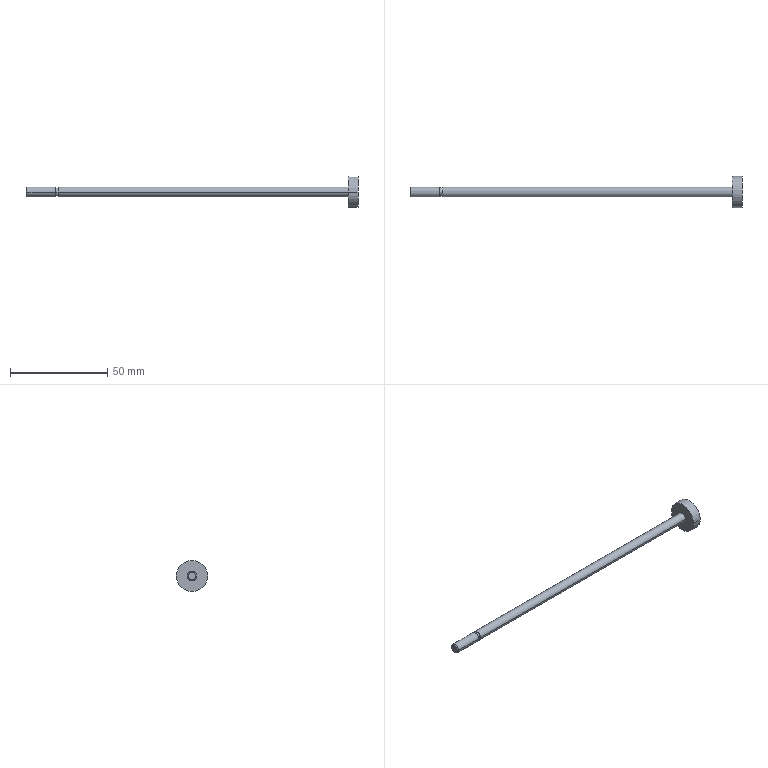Part | SolidWorks | features RefAxis 9, 3DProfileFeature 3, Revolution 1 | 1 solid | 15 faces | box 170.5 x 16 x 16 mm | volume 4244 mm3 | cylinder 8 | plane 5 | cone 2 | commonest cylinder face diameters 5 x4 4.134 x2 16 x2
STEP:
#1=CARTESIAN_POINT('',(170.5,-8.,0.));
#2=VERTEX_POINT('',#1);
#3=CARTESIAN_POINT('',(170.5,8.,0.));
#4=VERTEX_POINT('',#3);
#5=CARTESIAN_POINT('',(170.5,0.,0.));
#6=DIRECTION('',(-1.,0.,0.));
#7=DIRECTION('',(0.,-1.,0.));
#8=AXIS2_PLACEMENT_3D('',#5,#6,#7);
#9=CIRCLE('',#8,8.);
#10=EDGE_CURVE('',#2,#4,#9,.T.);
#11=ORIENTED_EDGE('',*,*,#10,.T.);
#12=CARTESIAN_POINT('',(165.5,8.,0.));
#13=VERTEX_POINT('',#12);
#14=CARTESIAN_POINT('',(170.5,8.,0.));
#15=DIRECTION('',(-1.,0.,0.));
#16=VECTOR('',#15,1000.);
#17=LINE('',#14,#16);
#18=EDGE_CURVE('',#4,#13,#17,.T.);
#19=ORIENTED_EDGE('',*,*,#18,.T.);
#20=CARTESIAN_POINT('',(165.5,-8.,0.));
#21=VERTEX_POINT('',#20);
#22=CARTESIAN_POINT('',(165.5,0.,0.));
#23=DIRECTION('',(-1.,0.,0.));
#24=DIRECTION('',(0.,-1.,0.));
#25=AXIS2_PLACEMENT_3D('',#22,#23,#24);
#26=CIRCLE('',#25,8.);
#27=EDGE_CURVE('',#21,#13,#26,.T.);
#28=ORIENTED_EDGE('',*,*,#27,.F.);
#29=CARTESIAN_POINT('',(170.5,-8.,0.));
#30=DIRECTION('',(-1.,0.,0.));
#31=VECTOR('',#30,1000.);
#32=LINE('',#29,#31);
#33=EDGE_CURVE('',#2,#21,#32,.T.);
#34=ORIENTED_EDGE('',*,*,#33,.F.);
#35=EDGE_LOOP('',(#11,#19,#28,#34));
#36=FACE_OUTER_BOUND('',#35,.T.);
#37=CARTESIAN_POINT('',(170.5,0.,0.));
#38=DIRECTION('',(-1.,0.,0.));
#39=DIRECTION('',(0.,-1.,0.));
#40=AXIS2_PLACEMENT_3D('',#37,#38,#39);
#41=CYLINDRICAL_SURFACE('',#40,8.);
#42=ADVANCED_FACE('',(#36),#41,.T.);
#43=CARTESIAN_POINT('',(165.5,-2.5,0.));
#44=VERTEX_POINT('',#43);
#45=CARTESIAN_POINT('',(165.5,2.5,0.));
#46=VERTEX_POINT('',#45);
#47=CARTESIAN_POINT('',(165.5,0.,0.));
#48=DIRECTION('',(-1.,0.,0.));
#49=DIRECTION('',(0.,-1.,0.));
#50=AXIS2_PLACEMENT_3D('',#47,#48,#49);
#51=CIRCLE('',#50,2.5);
#52=EDGE_CURVE('',#44,#46,#51,.T.);
#53=ORIENTED_EDGE('',*,*,#52,.T.);
#54=CARTESIAN_POINT('',(16.5,2.5,0.));
#55=VERTEX_POINT('',#54);
#56=CARTESIAN_POINT('',(170.5,2.5,0.));
#57=DIRECTION('',(-1.,0.,0.));
#58=VECTOR('',#57,1000.);
#59=LINE('',#56,#58);
#60=EDGE_CURVE('',#46,#55,#59,.T.);
#61=ORIENTED_EDGE('',*,*,#60,.T.);
#62=CARTESIAN_POINT('',(16.5,-2.5,0.));
#63=VERTEX_POINT('',#62);
#64=CARTESIAN_POINT('',(16.5,0.,0.));
#65=DIRECTION('',(-1.,0.,0.));
#66=DIRECTION('',(0.,-1.,0.));
#67=AXIS2_PLACEMENT_3D('',#64,#65,#66);
#68=CIRCLE('',#67,2.5);
#69=EDGE_CURVE('',#63,#55,#68,.T.);
#70=ORIENTED_EDGE('',*,*,#69,.F.);
#71=CARTESIAN_POINT('',(170.5,-2.5,0.));
#72=DIRECTION('',(-1.,0.,0.));
#73=VECTOR('',#72,1000.);
#74=LINE('',#71,#73);
#75=EDGE_CURVE('',#44,#63,#74,.T.);
#76=ORIENTED_EDGE('',*,*,#75,.F.);
#77=EDGE_LOOP('',(#53,#61,#70,#76));
#78=FACE_OUTER_BOUND('',#77,.T.);
#79=CARTESIAN_POINT('',(170.5,0.,0.));
#80=DIRECTION('',(-1.,0.,0.));
#81=DIRECTION('',(0.,-1.,0.));
#82=AXIS2_PLACEMENT_3D('',#79,#80,#81);
#83=CYLINDRICAL_SURFACE('',#82,2.5);
#84=ADVANCED_FACE('',(#78),#83,.T.);
#85=CARTESIAN_POINT('',(16.5,-2.067,0.));
#86=VERTEX_POINT('',#85);
#87=CARTESIAN_POINT('',(16.5,2.067,0.));
#88=VERTEX_POINT('',#87);
#89=CARTESIAN_POINT('',(16.5,0.,0.));
#90=DIRECTION('',(-1.,0.,0.));
#91=DIRECTION('',(0.,-1.,0.));
#92=AXIS2_PLACEMENT_3D('',#89,#90,#91);
#93=CIRCLE('',#92,2.067);
#94=EDGE_CURVE('',#86,#88,#93,.T.);
#95=ORIENTED_EDGE('',*,*,#94,.T.);
#96=CARTESIAN_POINT('',(15.,2.067,0.));
#97=VERTEX_POINT('',#96);
#98=CARTESIAN_POINT('',(170.5,2.067,0.));
#99=DIRECTION('',(-1.,0.,0.));
#100=VECTOR('',#99,1000.);
#101=LINE('',#98,#100);
#102=EDGE_CURVE('',#88,#97,#101,.T.);
#103=ORIENTED_EDGE('',*,*,#102,.T.);
#104=CARTESIAN_POINT('',(15.,-2.067,0.));
#105=VERTEX_POINT('',#104);
#106=CARTESIAN_POINT('',(15.,0.,0.));
#107=DIRECTION('',(-1.,0.,0.));
#108=DIRECTION('',(0.,-1.,0.));
#109=AXIS2_PLACEMENT_3D('',#106,#107,#108);
#110=CIRCLE('',#109,2.067);
#111=EDGE_CURVE('',#105,#97,#110,.T.);
#112=ORIENTED_EDGE('',*,*,#111,.F.);
#113=CARTESIAN_POINT('',(170.5,-2.067,0.));
#114=DIRECTION('',(-1.,0.,0.));
#115=VECTOR('',#114,1000.);
#116=LINE('',#113,#115);
#117=EDGE_CURVE('',#86,#105,#116,.T.);
#118=ORIENTED_EDGE('',*,*,#117,.F.);
#119=EDGE_LOOP('',(#95,#103,#112,#118));
#120=FACE_OUTER_BOUND('',#119,.T.);
#121=CARTESIAN_POINT('',(170.5,0.,0.));
#122=DIRECTION('',(-1.,0.,0.));
#123=DIRECTION('',(0.,-1.,0.));
#124=AXIS2_PLACEMENT_3D('',#121,#122,#123);
#125=CYLINDRICAL_SURFACE('',#124,2.067);
#126=ADVANCED_FACE('',(#120),#125,.T.);
#127=CARTESIAN_POINT('',(15.,-2.5,0.));
#128=VERTEX_POINT('',#127);
#129=CARTESIAN_POINT('',(15.,2.5,0.));
#130=VERTEX_POINT('',#129);
#131=CARTESIAN_POINT('',(15.,0.,0.));
#132=DIRECTION('',(-1.,0.,0.));
#133=DIRECTION('',(0.,-1.,0.));
#134=AXIS2_PLACEMENT_3D('',#131,#132,#133);
#135=CIRCLE('',#134,2.5);
#136=EDGE_CURVE('',#128,#130,#135,.T.);
#137=ORIENTED_EDGE('',*,*,#136,.T.);
#138=CARTESIAN_POINT('',(0.4905,2.5,0.));
#139=VERTEX_POINT('',#138);
#140=CARTESIAN_POINT('',(170.5,2.5,0.));
#141=DIRECTION('',(-1.,0.,0.));
#142=VECTOR('',#141,1000.);
#143=LINE('',#140,#142);
#144=EDGE_CURVE('',#130,#139,#143,.T.);
#145=ORIENTED_EDGE('',*,*,#144,.T.);
#146=CARTESIAN_POINT('',(0.4905,-2.5,0.));
#147=VERTEX_POINT('',#146);
#148=CARTESIAN_POINT('',(0.4905,0.,0.));
#149=DIRECTION('',(-1.,0.,0.));
#150=DIRECTION('',(0.,-1.,0.));
#151=AXIS2_PLACEMENT_3D('',#148,#149,#150);
#152=CIRCLE('',#151,2.5);
#153=EDGE_CURVE('',#147,#139,#152,.T.);
#154=ORIENTED_EDGE('',*,*,#153,.F.);
#155=CARTESIAN_POINT('',(170.5,-2.5,0.));
#156=DIRECTION('',(-1.,0.,0.));
#157=VECTOR('',#156,1000.);
#158=LINE('',#155,#157);
#159=EDGE_CURVE('',#128,#147,#158,.T.);
#160=ORIENTED_EDGE('',*,*,#159,.F.);
#161=EDGE_LOOP('',(#137,#145,#154,#160));
#162=FACE_OUTER_BOUND('',#161,.T.);
#163=CARTESIAN_POINT('',(170.5,0.,0.));
#164=DIRECTION('',(-1.,0.,0.));
#165=DIRECTION('',(0.,-1.,0.));
#166=AXIS2_PLACEMENT_3D('',#163,#164,#165);
#167=CYLINDRICAL_SURFACE('',#166,2.5);
#168=ADVANCED_FACE('',(#162),#167,.T.);
#169=CARTESIAN_POINT('',(0.,-2.01,0.));
#170=VERTEX_POINT('',#169);
#171=CARTESIAN_POINT('',(0.,2.01,0.));
#172=VERTEX_POINT('',#171);
#173=CARTESIAN_POINT('',(0.,0.,0.));
#174=DIRECTION('',(-1.,0.,0.));
#175=DIRECTION('',(0.,-1.,0.));
#176=AXIS2_PLACEMENT_3D('',#173,#174,#175);
#177=CIRCLE('',#176,2.01);
#178=EDGE_CURVE('',#170,#172,#177,.T.);
#179=ORIENTED_EDGE('',*,*,#178,.F.);
#180=CARTESIAN_POINT('',(0.4905,-2.5,0.));
#181=DIRECTION('',(0.7071,-0.7071,0.));
#182=VECTOR('',#181,1000.);
#183=LINE('',#180,#182);
#184=EDGE_CURVE('',#170,#147,#183,.T.);
#185=ORIENTED_EDGE('',*,*,#184,.T.);
#186=ORIENTED_EDGE('',*,*,#153,.T.);
#187=CARTESIAN_POINT('',(0.4905,2.5,0.));
#188=DIRECTION('',(0.7071,0.7071,0.));
#189=VECTOR('',#188,1000.);
#190=LINE('',#187,#189);
#191=EDGE_CURVE('',#172,#139,#190,.T.);
#192=ORIENTED_EDGE('',*,*,#191,.F.);
#193=EDGE_LOOP('',(#179,#185,#186,#192));
#194=FACE_OUTER_BOUND('',#193,.T.);
#195=CARTESIAN_POINT('',(0.4905,0.,0.));
#196=DIRECTION('',(1.,0.,0.));
#197=DIRECTION('',(0.,1.,0.));
#198=AXIS2_PLACEMENT_3D('',#195,#196,#197);
#199=CONICAL_SURFACE('',#198,2.5,0.7854);
#200=ADVANCED_FACE('',(#194),#199,.T.);
#201=CARTESIAN_POINT('',(0.,0.,0.));
#202=DIRECTION('',(-1.,0.,0.));
#203=DIRECTION('',(0.,-1.,0.));
#204=AXIS2_PLACEMENT_3D('',#201,#202,#203);
#205=CIRCLE('',#204,2.01);
#206=EDGE_CURVE('',#172,#170,#205,.T.);
#207=ORIENTED_EDGE('',*,*,#206,.T.);
#208=ORIENTED_EDGE('',*,*,#178,.T.);
#209=EDGE_LOOP('',(#207,#208));
#210=FACE_OUTER_BOUND('',#209,.T.);
#211=CARTESIAN_POINT('',(0.,0.,0.));
#212=DIRECTION('',(1.,0.,0.));
#213=DIRECTION('',(0.,1.,0.));
#214=AXIS2_PLACEMENT_3D('',#211,#212,#213);
#215=PLANE('',#214);
#216=ADVANCED_FACE('',(#210),#215,.F.);
#217=ORIENTED_EDGE('',*,*,#184,.F.);
#218=ORIENTED_EDGE('',*,*,#206,.F.);
#219=ORIENTED_EDGE('',*,*,#191,.T.);
#220=CARTESIAN_POINT('',(0.4905,0.,0.));
#221=DIRECTION('',(-1.,0.,0.));
#222=DIRECTION('',(0.,-1.,0.));
#223=AXIS2_PLACEMENT_3D('',#220,#221,#222);
#224=CIRCLE('',#223,2.5);
#225=EDGE_CURVE('',#139,#147,#224,.T.);
#226=ORIENTED_EDGE('',*,*,#225,.T.);
#227=EDGE_LOOP('',(#217,#218,#219,#226));
#228=FACE_OUTER_BOUND('',#227,.T.);
#229=CARTESIAN_POINT('',(0.4905,0.,0.));
#230=DIRECTION('',(1.,0.,0.));
#231=DIRECTION('',(0.,1.,0.));
#232=AXIS2_PLACEMENT_3D('',#229,#230,#231);
#233=CONICAL_SURFACE('',#232,2.5,0.7854);
#234=ADVANCED_FACE('',(#228),#233,.T.);
#235=ORIENTED_EDGE('',*,*,#144,.F.);
#236=CARTESIAN_POINT('',(15.,0.,0.));
#237=DIRECTION('',(-1.,0.,0.));
#238=DIRECTION('',(0.,-1.,0.));
#239=AXIS2_PLACEMENT_3D('',#236,#237,#238);
#240=CIRCLE('',#239,2.5);
#241=EDGE_CURVE('',#130,#128,#240,.T.);
#242=ORIENTED_EDGE('',*,*,#241,.T.);
#243=ORIENTED_EDGE('',*,*,#159,.T.);
#244=ORIENTED_EDGE('',*,*,#225,.F.);
#245=EDGE_LOOP('',(#235,#242,#243,#244));
#246=FACE_OUTER_BOUND('',#245,.T.);
#247=CARTESIAN_POINT('',(170.5,0.,0.));
#248=DIRECTION('',(-1.,0.,0.));
#249=DIRECTION('',(0.,-1.,0.));
#250=AXIS2_PLACEMENT_3D('',#247,#248,#249);
#251=CYLINDRICAL_SURFACE('',#250,2.5);
#252=ADVANCED_FACE('',(#246),#251,.T.);
#253=ORIENTED_EDGE('',*,*,#136,.F.);
#254=ORIENTED_EDGE('',*,*,#241,.F.);
#255=EDGE_LOOP('',(#253,#254));
#256=FACE_OUTER_BOUND('',#255,.T.);
#257=ORIENTED_EDGE('',*,*,#111,.T.);
#258=CARTESIAN_POINT('',(15.,0.,0.));
#259=DIRECTION('',(-1.,0.,0.));
#260=DIRECTION('',(0.,-1.,0.));
#261=AXIS2_PLACEMENT_3D('',#258,#259,#260);
#262=CIRCLE('',#261,2.067);
#263=EDGE_CURVE('',#97,#105,#262,.T.);
#264=ORIENTED_EDGE('',*,*,#263,.T.);
#265=EDGE_LOOP('',(#257,#264));
#266=FACE_BOUND('',#265,.T.);
#267=CARTESIAN_POINT('',(15.,2.5,0.));
#268=DIRECTION('',(-1.,0.,0.));
#269=DIRECTION('',(0.,-1.,0.));
#270=AXIS2_PLACEMENT_3D('',#267,#268,#269);
#271=PLANE('',#270);
#272=ADVANCED_FACE('',(#256,#266),#271,.F.);
#273=ORIENTED_EDGE('',*,*,#102,.F.);
#274=CARTESIAN_POINT('',(16.5,0.,0.));
#275=DIRECTION('',(-1.,0.,0.));
#276=DIRECTION('',(0.,-1.,0.));
#277=AXIS2_PLACEMENT_3D('',#274,#275,#276);
#278=CIRCLE('',#277,2.067);
#279=EDGE_CURVE('',#88,#86,#278,.T.);
#280=ORIENTED_EDGE('',*,*,#279,.T.);
#281=ORIENTED_EDGE('',*,*,#117,.T.);
#282=ORIENTED_EDGE('',*,*,#263,.F.);
#283=EDGE_LOOP('',(#273,#280,#281,#282));
#284=FACE_OUTER_BOUND('',#283,.T.);
#285=CARTESIAN_POINT('',(170.5,0.,0.));
#286=DIRECTION('',(-1.,0.,0.));
#287=DIRECTION('',(0.,-1.,0.));
#288=AXIS2_PLACEMENT_3D('',#285,#286,#287);
#289=CYLINDRICAL_SURFACE('',#288,2.067);
#290=ADVANCED_FACE('',(#284),#289,.T.);
#291=ORIENTED_EDGE('',*,*,#94,.F.);
#292=ORIENTED_EDGE('',*,*,#279,.F.);
#293=EDGE_LOOP('',(#291,#292));
#294=FACE_BOUND('',#293,.T.);
#295=ORIENTED_EDGE('',*,*,#69,.T.);
#296=CARTESIAN_POINT('',(16.5,0.,0.));
#297=DIRECTION('',(-1.,0.,0.));
#298=DIRECTION('',(0.,-1.,0.));
#299=AXIS2_PLACEMENT_3D('',#296,#297,#298);
#300=CIRCLE('',#299,2.5);
#301=EDGE_CURVE('',#55,#63,#300,.T.);
#302=ORIENTED_EDGE('',*,*,#301,.T.);
#303=EDGE_LOOP('',(#295,#302));
#304=FACE_OUTER_BOUND('',#303,.T.);
#305=CARTESIAN_POINT('',(16.5,2.067,0.));
#306=DIRECTION('',(1.,0.,0.));
#307=DIRECTION('',(0.,1.,0.));
#308=AXIS2_PLACEMENT_3D('',#305,#306,#307);
#309=PLANE('',#308);
#310=ADVANCED_FACE('',(#294,#304),#309,.F.);
#311=ORIENTED_EDGE('',*,*,#60,.F.);
#312=CARTESIAN_POINT('',(165.5,0.,0.));
#313=DIRECTION('',(-1.,0.,0.));
#314=DIRECTION('',(0.,-1.,0.));
#315=AXIS2_PLACEMENT_3D('',#312,#313,#314);
#316=CIRCLE('',#315,2.5);
#317=EDGE_CURVE('',#46,#44,#316,.T.);
#318=ORIENTED_EDGE('',*,*,#317,.T.);
#319=ORIENTED_EDGE('',*,*,#75,.T.);
#320=ORIENTED_EDGE('',*,*,#301,.F.);
#321=EDGE_LOOP('',(#311,#318,#319,#320));
#322=FACE_OUTER_BOUND('',#321,.T.);
#323=CARTESIAN_POINT('',(170.5,0.,0.));
#324=DIRECTION('',(-1.,0.,0.));
#325=DIRECTION('',(0.,-1.,0.));
#326=AXIS2_PLACEMENT_3D('',#323,#324,#325);
#327=CYLINDRICAL_SURFACE('',#326,2.5);
#328=ADVANCED_FACE('',(#322),#327,.T.);
#329=ORIENTED_EDGE('',*,*,#52,.F.);
#330=ORIENTED_EDGE('',*,*,#317,.F.);
#331=EDGE_LOOP('',(#329,#330));
#332=FACE_BOUND('',#331,.T.);
#333=ORIENTED_EDGE('',*,*,#27,.T.);
#334=CARTESIAN_POINT('',(165.5,0.,0.));
#335=DIRECTION('',(-1.,0.,0.));
#336=DIRECTION('',(0.,-1.,0.));
#337=AXIS2_PLACEMENT_3D('',#334,#335,#336);
#338=CIRCLE('',#337,8.);
#339=EDGE_CURVE('',#13,#21,#338,.T.);
#340=ORIENTED_EDGE('',*,*,#339,.T.);
#341=EDGE_LOOP('',(#333,#340));
#342=FACE_OUTER_BOUND('',#341,.T.);
#343=CARTESIAN_POINT('',(165.5,2.5,0.));
#344=DIRECTION('',(1.,0.,0.));
#345=DIRECTION('',(0.,1.,0.));
#346=AXIS2_PLACEMENT_3D('',#343,#344,#345);
#347=PLANE('',#346);
#348=ADVANCED_FACE('',(#332,#342),#347,.F.);
#349=ORIENTED_EDGE('',*,*,#18,.F.);
#350=CARTESIAN_POINT('',(170.5,0.,0.));
#351=DIRECTION('',(-1.,0.,0.));
#352=DIRECTION('',(0.,-1.,0.));
#353=AXIS2_PLACEMENT_3D('',#350,#351,#352);
#354=CIRCLE('',#353,8.);
#355=EDGE_CURVE('',#4,#2,#354,.T.);
#356=ORIENTED_EDGE('',*,*,#355,.T.);
#357=ORIENTED_EDGE('',*,*,#33,.T.);
#358=ORIENTED_EDGE('',*,*,#339,.F.);
#359=EDGE_LOOP('',(#349,#356,#357,#358));
#360=FACE_OUTER_BOUND('',#359,.T.);
#361=CARTESIAN_POINT('',(170.5,0.,0.));
#362=DIRECTION('',(-1.,0.,0.));
#363=DIRECTION('',(0.,-1.,0.));
#364=AXIS2_PLACEMENT_3D('',#361,#362,#363);
#365=CYLINDRICAL_SURFACE('',#364,8.);
#366=ADVANCED_FACE('',(#360),#365,.T.);
#367=ORIENTED_EDGE('',*,*,#10,.F.);
#368=ORIENTED_EDGE('',*,*,#355,.F.);
#369=EDGE_LOOP('',(#367,#368));
#370=FACE_OUTER_BOUND('',#369,.T.);
#371=CARTESIAN_POINT('',(170.5,8.,0.));
#372=DIRECTION('',(-1.,0.,0.));
#373=DIRECTION('',(0.,-1.,0.));
#374=AXIS2_PLACEMENT_3D('',#371,#372,#373);
#375=PLANE('',#374);
#376=ADVANCED_FACE('',(#370),#375,.F.);
#377=CLOSED_SHELL('',(#42,#84,#126,#168,#200,#216,#234,#252,#272,#290,#310,#328,#348,#366,#376));
#378=MANIFOLD_SOLID_BREP('',#377);
#379=CARTESIAN_POINT('',(0.,0.,0.));
#380=DIRECTION('',(0.,0.,1.));
#381=DIRECTION('',(1.,0.,0.));
#382=AXIS2_PLACEMENT_3D('',#379,#380,#381);
#383=(LENGTH_UNIT()NAMED_UNIT(*)SI_UNIT(.MILLI.,.METRE.));
#384=UNCERTAINTY_MEASURE_WITH_UNIT(LENGTH_MEASURE(0.00001),#383,'','');
#385=(NAMED_UNIT(*)PLANE_ANGLE_UNIT()SI_UNIT($,.RADIAN.));
#386=(NAMED_UNIT(*)SI_UNIT($,.STERADIAN.)SOLID_ANGLE_UNIT());
#387=(GEOMETRIC_REPRESENTATION_CONTEXT(3)GLOBAL_UNCERTAINTY_ASSIGNED_CONTEXT((#384))GLOBAL_UNIT_ASSIGNED_CONTEXT((#383,#385,#386))REPRESENTATION_CONTEXT('',''));
#388=ADVANCED_BREP_SHAPE_REPRESENTATION('',(#378,#382),#387);